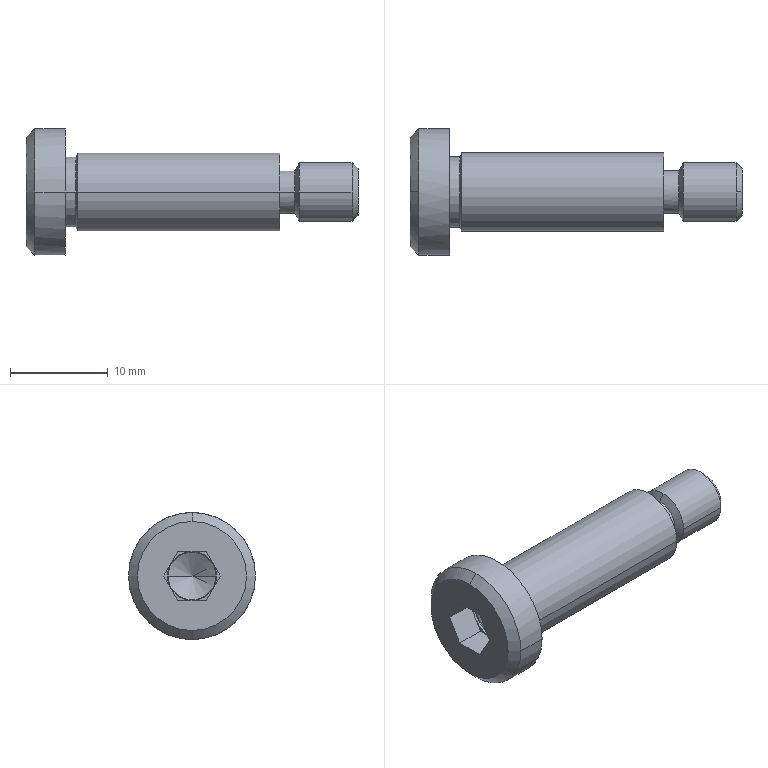Part | SolidWorks | features BaseBody 1 | 1 solid | 40 faces | box 34 x 13 x 13 mm | volume 1729 mm3 | plane 16 | cylinder 12 | cone 10 | spline 2 | commonest cylinder face diameters 4.4 x2 5 x2 6 x2 7.22 x2 8 x2 13 x2
STEP:
#1=CARTESIAN_POINT('',(-0.6825,-2.45,0.));
#2=VERTEX_POINT('',#1);
#3=CARTESIAN_POINT('',(-0.6825,2.45,0.));
#4=VERTEX_POINT('',#3);
#5=CARTESIAN_POINT('',(-0.6825,0.,0.));
#6=DIRECTION('',(-1.,0.,0.));
#7=DIRECTION('',(0.,1.,0.));
#8=AXIS2_PLACEMENT_3D('',#5,#6,#7);
#9=CIRCLE('',#8,2.45);
#10=EDGE_CURVE('',#2,#4,#9,.T.);
#11=ORIENTED_EDGE('',*,*,#10,.F.);
#12=CARTESIAN_POINT('',(-0.7691,-2.5,0.));
#13=VERTEX_POINT('',#12);
#14=CARTESIAN_POINT('',(-0.7691,-2.4,0.));
#15=DIRECTION('',(0.,0.,-1.));
#16=DIRECTION('',(0.,-1.,0.));
#17=AXIS2_PLACEMENT_3D('',#14,#15,#16);
#18=CIRCLE('',#17,0.1);
#19=EDGE_CURVE('',#2,#13,#18,.T.);
#20=ORIENTED_EDGE('',*,*,#19,.T.);
#21=CARTESIAN_POINT('',(-0.7691,2.5,0.));
#22=VERTEX_POINT('',#21);
#23=CARTESIAN_POINT('',(-0.7691,0.,0.));
#24=DIRECTION('',(-1.,0.,0.));
#25=DIRECTION('',(0.,1.,0.));
#26=AXIS2_PLACEMENT_3D('',#23,#24,#25);
#27=CIRCLE('',#26,2.5);
#28=EDGE_CURVE('',#13,#22,#27,.T.);
#29=ORIENTED_EDGE('',*,*,#28,.T.);
#30=CARTESIAN_POINT('',(-0.7691,2.4,0.));
#31=DIRECTION('',(0.,0.,1.));
#32=DIRECTION('',(0.,1.,0.));
#33=AXIS2_PLACEMENT_3D('',#30,#31,#32);
#34=CIRCLE('',#33,0.1);
#35=EDGE_CURVE('',#4,#22,#34,.T.);
#36=ORIENTED_EDGE('',*,*,#35,.F.);
#37=EDGE_LOOP('',(#11,#20,#29,#36));
#38=FACE_OUTER_BOUND('',#37,.T.);
#39=CARTESIAN_POINT('',(-0.6825,2.45,0.));
#40=CARTESIAN_POINT('',(-0.6825,2.45,4.9));
#41=CARTESIAN_POINT('',(-0.6825,-2.45,4.9));
#42=CARTESIAN_POINT('',(-0.6825,-2.45,0.));
#43=CARTESIAN_POINT('',(-0.7008,2.482,0.));
#44=CARTESIAN_POINT('',(-0.7008,2.482,4.963));
#45=CARTESIAN_POINT('',(-0.7008,-2.482,4.963));
#46=CARTESIAN_POINT('',(-0.7008,-2.482,0.));
#47=CARTESIAN_POINT('',(-0.7325,2.5,0.));
#48=CARTESIAN_POINT('',(-0.7325,2.5,5.));
#49=CARTESIAN_POINT('',(-0.7325,-2.5,5.));
#50=CARTESIAN_POINT('',(-0.7325,-2.5,0.));
#51=CARTESIAN_POINT('',(-0.7691,2.5,0.));
#52=CARTESIAN_POINT('',(-0.7691,2.5,5.));
#53=CARTESIAN_POINT('',(-0.7691,-2.5,5.));
#54=CARTESIAN_POINT('',(-0.7691,-2.5,0.));
#55=(BOUNDED_SURFACE()B_SPLINE_SURFACE(3,3,((#39,#40,#41,#42),(#43,#44,#45,#46),(#47,#48,#49,#50),(#51,#52,#53,#54)),.UNSPECIFIED.,.F.,.F.,.F.)B_SPLINE_SURFACE_WITH_KNOTS((4,4),(4,4),(0.,1.),(0.,1.),.UNSPECIFIED.)GEOMETRIC_REPRESENTATION_ITEM()RATIONAL_B_SPLINE_SURFACE(((1.,0.3333,0.3333,1.),(0.9107,0.3036,0.3036,0.9107),(0.9107,0.3036,0.3036,0.9107),(1.,0.3333,0.3333,1.)))REPRESENTATION_ITEM('')SURFACE());
#56=ADVANCED_FACE('',(#38),#55,.F.);
#57=CARTESIAN_POINT('',(1.3,4.,0.));
#58=VERTEX_POINT('',#57);
#59=CARTESIAN_POINT('',(1.3,-4.,0.));
#60=VERTEX_POINT('',#59);
#61=CARTESIAN_POINT('',(1.3,0.,0.));
#62=DIRECTION('',(1.,0.,0.));
#63=DIRECTION('',(0.,1.,0.));
#64=AXIS2_PLACEMENT_3D('',#61,#62,#63);
#65=CIRCLE('',#64,4.);
#66=EDGE_CURVE('',#58,#60,#65,.T.);
#67=ORIENTED_EDGE('',*,*,#66,.T.);
#68=CARTESIAN_POINT('',(22.,-4.,0.));
#69=VERTEX_POINT('',#68);
#70=CARTESIAN_POINT('',(500.,-4.,0.));
#71=DIRECTION('',(1.,0.,0.));
#72=VECTOR('',#71,1000.);
#73=LINE('',#70,#72);
#74=EDGE_CURVE('',#60,#69,#73,.T.);
#75=ORIENTED_EDGE('',*,*,#74,.T.);
#76=CARTESIAN_POINT('',(22.,4.,0.));
#77=VERTEX_POINT('',#76);
#78=CARTESIAN_POINT('',(22.,0.,0.));
#79=DIRECTION('',(-1.,0.,0.));
#80=DIRECTION('',(0.,1.,0.));
#81=AXIS2_PLACEMENT_3D('',#78,#79,#80);
#82=CIRCLE('',#81,4.);
#83=EDGE_CURVE('',#69,#77,#82,.T.);
#84=ORIENTED_EDGE('',*,*,#83,.T.);
#85=CARTESIAN_POINT('',(500.,4.,0.));
#86=DIRECTION('',(1.,0.,0.));
#87=VECTOR('',#86,1000.);
#88=LINE('',#85,#87);
#89=EDGE_CURVE('',#58,#77,#88,.T.);
#90=ORIENTED_EDGE('',*,*,#89,.F.);
#91=EDGE_LOOP('',(#67,#75,#84,#90));
#92=FACE_OUTER_BOUND('',#91,.T.);
#93=CARTESIAN_POINT('',(500.,0.,0.));
#94=DIRECTION('',(1.,0.,0.));
#95=DIRECTION('',(0.,1.,0.));
#96=AXIS2_PLACEMENT_3D('',#93,#94,#95);
#97=CYLINDRICAL_SURFACE('',#96,4.);
#98=ADVANCED_FACE('',(#92),#97,.T.);
#99=CARTESIAN_POINT('',(1.075,3.61,0.));
#100=VERTEX_POINT('',#99);
#101=CARTESIAN_POINT('',(1.075,-3.61,0.));
#102=VERTEX_POINT('',#101);
#103=CARTESIAN_POINT('',(1.075,0.,0.));
#104=DIRECTION('',(1.,0.,0.));
#105=DIRECTION('',(0.,1.,0.));
#106=AXIS2_PLACEMENT_3D('',#103,#104,#105);
#107=CIRCLE('',#106,3.61);
#108=EDGE_CURVE('',#100,#102,#107,.T.);
#109=ORIENTED_EDGE('',*,*,#108,.T.);
#110=CARTESIAN_POINT('',(1.3,-4.,0.));
#111=DIRECTION('',(0.5,-0.866,0.));
#112=VECTOR('',#111,1000.);
#113=LINE('',#110,#112);
#114=EDGE_CURVE('',#102,#60,#113,.T.);
#115=ORIENTED_EDGE('',*,*,#114,.T.);
#116=ORIENTED_EDGE('',*,*,#66,.F.);
#117=CARTESIAN_POINT('',(1.3,4.,0.));
#118=DIRECTION('',(0.5,0.866,0.));
#119=VECTOR('',#118,1000.);
#120=LINE('',#117,#119);
#121=EDGE_CURVE('',#100,#58,#120,.T.);
#122=ORIENTED_EDGE('',*,*,#121,.F.);
#123=EDGE_LOOP('',(#109,#115,#116,#122));
#124=FACE_OUTER_BOUND('',#123,.T.);
#125=CARTESIAN_POINT('',(1.3,0.,0.));
#126=DIRECTION('',(1.,0.,0.));
#127=DIRECTION('',(0.,1.,0.));
#128=AXIS2_PLACEMENT_3D('',#125,#126,#127);
#129=CONICAL_SURFACE('',#128,4.,1.047);
#130=ADVANCED_FACE('',(#124),#129,.T.);
#131=CARTESIAN_POINT('',(0.,3.61,0.));
#132=VERTEX_POINT('',#131);
#133=CARTESIAN_POINT('',(0.,-3.61,0.));
#134=VERTEX_POINT('',#133);
#135=CARTESIAN_POINT('',(0.,0.,0.));
#136=DIRECTION('',(1.,0.,0.));
#137=DIRECTION('',(0.,1.,0.));
#138=AXIS2_PLACEMENT_3D('',#135,#136,#137);
#139=CIRCLE('',#138,3.61);
#140=EDGE_CURVE('',#132,#134,#139,.T.);
#141=ORIENTED_EDGE('',*,*,#140,.T.);
#142=CARTESIAN_POINT('',(500.,-3.61,0.));
#143=DIRECTION('',(1.,0.,0.));
#144=VECTOR('',#143,1000.);
#145=LINE('',#142,#144);
#146=EDGE_CURVE('',#134,#102,#145,.T.);
#147=ORIENTED_EDGE('',*,*,#146,.T.);
#148=ORIENTED_EDGE('',*,*,#108,.F.);
#149=CARTESIAN_POINT('',(500.,3.61,0.));
#150=DIRECTION('',(1.,0.,0.));
#151=VECTOR('',#150,1000.);
#152=LINE('',#149,#151);
#153=EDGE_CURVE('',#132,#100,#152,.T.);
#154=ORIENTED_EDGE('',*,*,#153,.F.);
#155=EDGE_LOOP('',(#141,#147,#148,#154));
#156=FACE_OUTER_BOUND('',#155,.T.);
#157=CARTESIAN_POINT('',(500.,0.,0.));
#158=DIRECTION('',(1.,0.,0.));
#159=DIRECTION('',(0.,1.,0.));
#160=AXIS2_PLACEMENT_3D('',#157,#158,#159);
#161=CYLINDRICAL_SURFACE('',#160,3.61);
#162=ADVANCED_FACE('',(#156),#161,.T.);
#163=CARTESIAN_POINT('',(22.,2.2,0.));
#164=VERTEX_POINT('',#163);
#165=CARTESIAN_POINT('',(22.,-2.2,0.));
#166=VERTEX_POINT('',#165);
#167=CARTESIAN_POINT('',(22.,0.,0.));
#168=DIRECTION('',(1.,0.,0.));
#169=DIRECTION('',(0.,1.,0.));
#170=AXIS2_PLACEMENT_3D('',#167,#168,#169);
#171=CIRCLE('',#170,2.2);
#172=EDGE_CURVE('',#164,#166,#171,.T.);
#173=ORIENTED_EDGE('',*,*,#172,.T.);
#174=CARTESIAN_POINT('',(23.538,-2.2,0.));
#175=VERTEX_POINT('',#174);
#176=CARTESIAN_POINT('',(500.,-2.2,0.));
#177=DIRECTION('',(1.,0.,0.));
#178=VECTOR('',#177,1000.);
#179=LINE('',#176,#178);
#180=EDGE_CURVE('',#166,#175,#179,.T.);
#181=ORIENTED_EDGE('',*,*,#180,.T.);
#182=CARTESIAN_POINT('',(23.538,0.,2.2));
#183=VERTEX_POINT('',#182);
#184=CARTESIAN_POINT('',(23.538,0.,0.));
#185=DIRECTION('',(-1.,0.,0.));
#186=DIRECTION('',(0.,1.,0.));
#187=AXIS2_PLACEMENT_3D('',#184,#185,#186);
#188=CIRCLE('',#187,2.2);
#189=EDGE_CURVE('',#175,#183,#188,.T.);
#190=ORIENTED_EDGE('',*,*,#189,.T.);
#191=CARTESIAN_POINT('',(23.538,2.2,0.));
#192=VERTEX_POINT('',#191);
#193=CARTESIAN_POINT('',(23.538,0.,0.));
#194=DIRECTION('',(-1.,0.,0.));
#195=DIRECTION('',(0.,1.,0.));
#196=AXIS2_PLACEMENT_3D('',#193,#194,#195);
#197=CIRCLE('',#196,2.2);
#198=EDGE_CURVE('',#183,#192,#197,.T.);
#199=ORIENTED_EDGE('',*,*,#198,.T.);
#200=CARTESIAN_POINT('',(500.,2.2,0.));
#201=DIRECTION('',(1.,0.,0.));
#202=VECTOR('',#201,1000.);
#203=LINE('',#200,#202);
#204=EDGE_CURVE('',#164,#192,#203,.T.);
#205=ORIENTED_EDGE('',*,*,#204,.F.);
#206=EDGE_LOOP('',(#173,#181,#190,#199,#205));
#207=FACE_OUTER_BOUND('',#206,.T.);
#208=CARTESIAN_POINT('',(500.,0.,0.));
#209=DIRECTION('',(1.,0.,0.));
#210=DIRECTION('',(0.,1.,0.));
#211=AXIS2_PLACEMENT_3D('',#208,#209,#210);
#212=CYLINDRICAL_SURFACE('',#211,2.2);
#213=ADVANCED_FACE('',(#207),#212,.T.);
#214=ORIENTED_EDGE('',*,*,#198,.F.);
#215=CARTESIAN_POINT('',(24.,0.,3.));
#216=VERTEX_POINT('',#215);
#217=CARTESIAN_POINT('',(24.,0.,3.));
#218=DIRECTION('',(0.5,0.,0.866));
#219=VECTOR('',#218,1000.);
#220=LINE('',#217,#219);
#221=EDGE_CURVE('',#183,#216,#220,.T.);
#222=ORIENTED_EDGE('',*,*,#221,.T.);
#223=CARTESIAN_POINT('',(24.,3.,0.));
#224=VERTEX_POINT('',#223);
#225=CARTESIAN_POINT('',(24.,0.,0.));
#226=DIRECTION('',(-1.,0.,0.));
#227=DIRECTION('',(0.,1.,0.));
#228=AXIS2_PLACEMENT_3D('',#225,#226,#227);
#229=CIRCLE('',#228,3.);
#230=EDGE_CURVE('',#216,#224,#229,.T.);
#231=ORIENTED_EDGE('',*,*,#230,.T.);
#232=CARTESIAN_POINT('',(24.,0.,-3.));
#233=VERTEX_POINT('',#232);
#234=CARTESIAN_POINT('',(24.,0.,0.));
#235=DIRECTION('',(-1.,0.,0.));
#236=DIRECTION('',(0.,1.,0.));
#237=AXIS2_PLACEMENT_3D('',#234,#235,#236);
#238=CIRCLE('',#237,3.);
#239=EDGE_CURVE('',#224,#233,#238,.T.);
#240=ORIENTED_EDGE('',*,*,#239,.T.);
#241=CARTESIAN_POINT('',(23.538,0.,-2.2));
#242=VERTEX_POINT('',#241);
#243=CARTESIAN_POINT('',(24.,0.,-3.));
#244=DIRECTION('',(0.5,0.,-0.866));
#245=VECTOR('',#244,1000.);
#246=LINE('',#243,#245);
#247=EDGE_CURVE('',#242,#233,#246,.T.);
#248=ORIENTED_EDGE('',*,*,#247,.F.);
#249=CARTESIAN_POINT('',(23.538,0.,0.));
#250=DIRECTION('',(-1.,0.,0.));
#251=DIRECTION('',(0.,1.,0.));
#252=AXIS2_PLACEMENT_3D('',#249,#250,#251);
#253=CIRCLE('',#252,2.2);
#254=EDGE_CURVE('',#192,#242,#253,.T.);
#255=ORIENTED_EDGE('',*,*,#254,.F.);
#256=EDGE_LOOP('',(#214,#222,#231,#240,#248,#255));
#257=FACE_OUTER_BOUND('',#256,.T.);
#258=CARTESIAN_POINT('',(24.,0.,0.));
#259=DIRECTION('',(1.,0.,0.));
#260=DIRECTION('',(0.,0.,-1.));
#261=AXIS2_PLACEMENT_3D('',#258,#259,#260);
#262=CONICAL_SURFACE('',#261,3.,1.047);
#263=ADVANCED_FACE('',(#257),#262,.T.);
#264=CARTESIAN_POINT('',(-3.081,0.,6.5));
#265=VERTEX_POINT('',#264);
#266=CARTESIAN_POINT('',(-3.081,-6.5,0.));
#267=VERTEX_POINT('',#266);
#268=CARTESIAN_POINT('',(-3.081,0.,0.));
#269=DIRECTION('',(1.,0.,0.));
#270=DIRECTION('',(0.,1.,0.));
#271=AXIS2_PLACEMENT_3D('',#268,#269,#270);
#272=CIRCLE('',#271,6.5);
#273=EDGE_CURVE('',#265,#267,#272,.T.);
#274=ORIENTED_EDGE('',*,*,#273,.T.);
#275=CARTESIAN_POINT('',(0.,-6.5,0.));
#276=VERTEX_POINT('',#275);
#277=CARTESIAN_POINT('',(500.,-6.5,0.));
#278=DIRECTION('',(1.,0.,0.));
#279=VECTOR('',#278,1000.);
#280=LINE('',#277,#279);
#281=EDGE_CURVE('',#267,#276,#280,.T.);
#282=ORIENTED_EDGE('',*,*,#281,.T.);
#283=CARTESIAN_POINT('',(0.,6.5,0.));
#284=VERTEX_POINT('',#283);
#285=CARTESIAN_POINT('',(0.,0.,0.));
#286=DIRECTION('',(-1.,0.,0.));
#287=DIRECTION('',(0.,1.,0.));
#288=AXIS2_PLACEMENT_3D('',#285,#286,#287);
#289=CIRCLE('',#288,6.5);
#290=EDGE_CURVE('',#276,#284,#289,.T.);
#291=ORIENTED_EDGE('',*,*,#290,.T.);
#292=CARTESIAN_POINT('',(-3.081,6.5,0.));
#293=VERTEX_POINT('',#292);
#294=CARTESIAN_POINT('',(500.,6.5,0.));
#295=DIRECTION('',(1.,0.,0.));
#296=VECTOR('',#295,1000.);
#297=LINE('',#294,#296);
#298=EDGE_CURVE('',#293,#284,#297,.T.);
#299=ORIENTED_EDGE('',*,*,#298,.F.);
#300=CARTESIAN_POINT('',(-3.081,0.,0.));
#301=DIRECTION('',(1.,0.,0.));
#302=DIRECTION('',(0.,1.,0.));
#303=AXIS2_PLACEMENT_3D('',#300,#301,#302);
#304=CIRCLE('',#303,6.5);
#305=EDGE_CURVE('',#293,#265,#304,.T.);
#306=ORIENTED_EDGE('',*,*,#305,.T.);
#307=EDGE_LOOP('',(#274,#282,#291,#299,#306));
#308=FACE_OUTER_BOUND('',#307,.T.);
#309=CARTESIAN_POINT('',(500.,0.,0.));
#310=DIRECTION('',(1.,0.,0.));
#311=DIRECTION('',(0.,1.,0.));
#312=AXIS2_PLACEMENT_3D('',#309,#310,#311);
#313=CYLINDRICAL_SURFACE('',#312,6.5);
#314=ADVANCED_FACE('',(#308),#313,.T.);
#315=CARTESIAN_POINT('',(24.,-3.,0.));
#316=VERTEX_POINT('',#315);
#317=CARTESIAN_POINT('',(24.,0.,0.));
#318=DIRECTION('',(-1.,0.,0.));
#319=DIRECTION('',(0.,1.,0.));
#320=AXIS2_PLACEMENT_3D('',#317,#318,#319);
#321=CIRCLE('',#320,3.);
#322=EDGE_CURVE('',#316,#216,#321,.T.);
#323=ORIENTED_EDGE('',*,*,#322,.F.);
#324=CARTESIAN_POINT('',(29.386,-3.,0.));
#325=VERTEX_POINT('',#324);
#326=CARTESIAN_POINT('',(500.,-3.,0.));
#327=DIRECTION('',(1.,0.,0.));
#328=VECTOR('',#327,1000.);
#329=LINE('',#326,#328);
#330=EDGE_CURVE('',#316,#325,#329,.T.);
#331=ORIENTED_EDGE('',*,*,#330,.T.);
#332=CARTESIAN_POINT('',(29.386,0.,3.));
#333=VERTEX_POINT('',#332);
#334=CARTESIAN_POINT('',(29.386,0.,0.));
#335=DIRECTION('',(-1.,0.,0.));
#336=DIRECTION('',(0.,1.,0.));
#337=AXIS2_PLACEMENT_3D('',#334,#335,#336);
#338=CIRCLE('',#337,3.);
#339=EDGE_CURVE('',#325,#333,#338,.T.);
#340=ORIENTED_EDGE('',*,*,#339,.T.);
#341=CARTESIAN_POINT('',(29.386,3.,0.));
#342=VERTEX_POINT('',#341);
#343=CARTESIAN_POINT('',(29.386,0.,0.));
#344=DIRECTION('',(-1.,0.,0.));
#345=DIRECTION('',(0.,1.,0.));
#346=AXIS2_PLACEMENT_3D('',#343,#344,#345);
#347=CIRCLE('',#346,3.);
#348=EDGE_CURVE('',#333,#342,#347,.T.);
#349=ORIENTED_EDGE('',*,*,#348,.T.);
#350=CARTESIAN_POINT('',(500.,3.,0.));
#351=DIRECTION('',(1.,0.,0.));
#352=VECTOR('',#351,1000.);
#353=LINE('',#350,#352);
#354=EDGE_CURVE('',#224,#342,#353,.T.);
#355=ORIENTED_EDGE('',*,*,#354,.F.);
#356=ORIENTED_EDGE('',*,*,#230,.F.);
#357=EDGE_LOOP('',(#323,#331,#340,#349,#355,#356));
#358=FACE_OUTER_BOUND('',#357,.T.);
#359=CARTESIAN_POINT('',(500.,0.,0.));
#360=DIRECTION('',(1.,0.,0.));
#361=DIRECTION('',(0.,1.,0.));
#362=AXIS2_PLACEMENT_3D('',#359,#360,#361);
#363=CYLINDRICAL_SURFACE('',#362,3.);
#364=ADVANCED_FACE('',(#358),#363,.T.);
#365=CARTESIAN_POINT('',(-4.,0.,-5.581));
#366=VERTEX_POINT('',#365);
#367=CARTESIAN_POINT('',(-4.,0.,5.581));
#368=VERTEX_POINT('',#367);
#369=CARTESIAN_POINT('',(-4.,0.,0.));
#370=DIRECTION('',(1.,0.,0.));
#371=DIRECTION('',(0.,0.,-1.));
#372=AXIS2_PLACEMENT_3D('',#369,#370,#371);
#373=CIRCLE('',#372,5.581);
#374=EDGE_CURVE('',#366,#368,#373,.T.);
#375=ORIENTED_EDGE('',*,*,#374,.T.);
#376=CARTESIAN_POINT('',(-3.081,0.,6.5));
#377=DIRECTION('',(0.7071,0.,0.7071));
#378=VECTOR('',#377,1000.);
#379=LINE('',#376,#378);
#380=EDGE_CURVE('',#368,#265,#379,.T.);
#381=ORIENTED_EDGE('',*,*,#380,.T.);
#382=ORIENTED_EDGE('',*,*,#305,.F.);
#383=CARTESIAN_POINT('',(-3.081,0.,-6.5));
#384=VERTEX_POINT('',#383);
#385=CARTESIAN_POINT('',(-3.081,0.,0.));
#386=DIRECTION('',(1.,0.,0.));
#387=DIRECTION('',(0.,1.,0.));
#388=AXIS2_PLACEMENT_3D('',#385,#386,#387);
#389=CIRCLE('',#388,6.5);
#390=EDGE_CURVE('',#384,#293,#389,.T.);
#391=ORIENTED_EDGE('',*,*,#390,.F.);
#392=CARTESIAN_POINT('',(-3.081,0.,-6.5));
#393=DIRECTION('',(0.7071,0.,-0.7071));
#394=VECTOR('',#393,1000.);
#395=LINE('',#392,#394);
#396=EDGE_CURVE('',#366,#384,#395,.T.);
#397=ORIENTED_EDGE('',*,*,#396,.F.);
#398=EDGE_LOOP('',(#375,#381,#382,#391,#397));
#399=FACE_OUTER_BOUND('',#398,.T.);
#400=CARTESIAN_POINT('',(-3.081,0.,0.));
#401=DIRECTION('',(1.,0.,0.));
#402=DIRECTION('',(0.,0.,-1.));
#403=AXIS2_PLACEMENT_3D('',#400,#401,#402);
#404=CONICAL_SURFACE('',#403,6.5,0.7854);
#405=ADVANCED_FACE('',(#399),#404,.T.);
#406=CARTESIAN_POINT('',(30.,0.,2.387));
#407=VERTEX_POINT('',#406);
#408=CARTESIAN_POINT('',(30.,0.,-2.387));
#409=VERTEX_POINT('',#408);
#410=CARTESIAN_POINT('',(30.,0.,0.));
#411=DIRECTION('',(-1.,0.,0.));
#412=DIRECTION('',(0.,0.,1.));
#413=AXIS2_PLACEMENT_3D('',#410,#411,#412);
#414=CIRCLE('',#413,2.387);
#415=EDGE_CURVE('',#407,#409,#414,.T.);
#416=ORIENTED_EDGE('',*,*,#415,.T.);
#417=CARTESIAN_POINT('',(29.386,0.,-3.));
#418=VERTEX_POINT('',#417);
#419=CARTESIAN_POINT('',(29.387,0.,-3.));
#420=DIRECTION('',(-0.7071,0.,-0.7071));
#421=VECTOR('',#420,1000.);
#422=LINE('',#419,#421);
#423=EDGE_CURVE('',#409,#418,#422,.T.);
#424=ORIENTED_EDGE('',*,*,#423,.T.);
#425=CARTESIAN_POINT('',(29.386,0.,0.));
#426=DIRECTION('',(-1.,0.,0.));
#427=DIRECTION('',(0.,1.,0.));
#428=AXIS2_PLACEMENT_3D('',#425,#426,#427);
#429=CIRCLE('',#428,3.);
#430=EDGE_CURVE('',#342,#418,#429,.T.);
#431=ORIENTED_EDGE('',*,*,#430,.F.);
#432=ORIENTED_EDGE('',*,*,#348,.F.);
#433=CARTESIAN_POINT('',(29.387,0.,3.));
#434=DIRECTION('',(-0.7071,0.,0.7071));
#435=VECTOR('',#434,1000.);
#436=LINE('',#433,#435);
#437=EDGE_CURVE('',#407,#333,#436,.T.);
#438=ORIENTED_EDGE('',*,*,#437,.F.);
#439=EDGE_LOOP('',(#416,#424,#431,#432,#438));
#440=FACE_OUTER_BOUND('',#439,.T.);
#441=CARTESIAN_POINT('',(29.387,0.,0.));
#442=DIRECTION('',(-1.,0.,0.));
#443=DIRECTION('',(0.,0.,1.));
#444=AXIS2_PLACEMENT_3D('',#441,#442,#443);
#445=CONICAL_SURFACE('',#444,3.,0.7854);
#446=ADVANCED_FACE('',(#440),#445,.T.);
#447=CARTESIAN_POINT('',(-1.,-2.5,0.));
#448=VERTEX_POINT('',#447);
#449=CARTESIAN_POINT('',(-1.,-2.165,-1.25));
#450=VERTEX_POINT('',#449);
#451=CARTESIAN_POINT('',(-1.,0.,0.));
#452=DIRECTION('',(1.,0.,0.));
#453=DIRECTION('',(0.,1.,0.));
#454=AXIS2_PLACEMENT_3D('',#451,#452,#453);
#455=CIRCLE('',#454,2.5);
#456=EDGE_CURVE('',#448,#450,#455,.T.);
#457=ORIENTED_EDGE('',*,*,#456,.F.);
#458=CARTESIAN_POINT('',(500.,-2.5,0.));
#459=DIRECTION('',(1.,0.,0.));
#460=VECTOR('',#459,1000.);
#461=LINE('',#458,#460);
#462=EDGE_CURVE('',#448,#13,#461,.T.);
#463=ORIENTED_EDGE('',*,*,#462,.T.);
#464=CARTESIAN_POINT('',(-0.7691,0.,0.));
#465=DIRECTION('',(-1.,0.,0.));
#466=DIRECTION('',(0.,1.,0.));
#467=AXIS2_PLACEMENT_3D('',#464,#465,#466);
#468=CIRCLE('',#467,2.5);
#469=EDGE_CURVE('',#22,#13,#468,.T.);
#470=ORIENTED_EDGE('',*,*,#469,.F.);
#471=CARTESIAN_POINT('',(-1.,2.5,0.));
#472=VERTEX_POINT('',#471);
#473=CARTESIAN_POINT('',(500.,2.5,0.));
#474=DIRECTION('',(1.,0.,0.));
#475=VECTOR('',#474,1000.);
#476=LINE('',#473,#475);
#477=EDGE_CURVE('',#472,#22,#476,.T.);
#478=ORIENTED_EDGE('',*,*,#477,.F.);
#479=CARTESIAN_POINT('',(-1.,2.165,-1.25));
#480=VERTEX_POINT('',#479);
#481=CARTESIAN_POINT('',(-1.,0.,0.));
#482=DIRECTION('',(1.,0.,0.));
#483=DIRECTION('',(0.,1.,0.));
#484=AXIS2_PLACEMENT_3D('',#481,#482,#483);
#485=CIRCLE('',#484,2.5);
#486=EDGE_CURVE('',#480,#472,#485,.T.);
#487=ORIENTED_EDGE('',*,*,#486,.F.);
#488=CARTESIAN_POINT('',(-1.,0.,-2.5));
#489=VERTEX_POINT('',#488);
#490=CARTESIAN_POINT('',(-1.,0.,0.));
#491=DIRECTION('',(1.,0.,0.));
#492=DIRECTION('',(0.,1.,0.));
#493=AXIS2_PLACEMENT_3D('',#490,#491,#492);
#494=CIRCLE('',#493,2.5);
#495=EDGE_CURVE('',#489,#480,#494,.T.);
#496=ORIENTED_EDGE('',*,*,#495,.F.);
#497=CARTESIAN_POINT('',(-1.,0.,0.));
#498=DIRECTION('',(1.,0.,0.));
#499=DIRECTION('',(0.,1.,0.));
#500=AXIS2_PLACEMENT_3D('',#497,#498,#499);
#501=CIRCLE('',#500,2.5);
#502=EDGE_CURVE('',#450,#489,#501,.T.);
#503=ORIENTED_EDGE('',*,*,#502,.F.);
#504=EDGE_LOOP('',(#457,#463,#470,#478,#487,#496,#503));
#505=FACE_OUTER_BOUND('',#504,.T.);
#506=CARTESIAN_POINT('',(500.,0.,0.));
#507=DIRECTION('',(1.,0.,0.));
#508=DIRECTION('',(0.,1.,0.));
#509=AXIS2_PLACEMENT_3D('',#506,#507,#508);
#510=CYLINDRICAL_SURFACE('',#509,2.5);
#511=ADVANCED_FACE('',(#505),#510,.F.);
#512=CARTESIAN_POINT('',(0.7321,0.,0.));
#513=VERTEX_POINT('',#512);
#514=CARTESIAN_POINT('',(-0.6825,-2.45,0.));
#515=DIRECTION('',(-0.5,-0.866,0.));
#516=VECTOR('',#515,1000.);
#517=LINE('',#514,#516);
#518=EDGE_CURVE('',#513,#2,#517,.T.);
#519=ORIENTED_EDGE('',*,*,#518,.F.);
#520=CARTESIAN_POINT('',(-0.6825,2.45,0.));
#521=DIRECTION('',(-0.5,0.866,0.));
#522=VECTOR('',#521,1000.);
#523=LINE('',#520,#522);
#524=EDGE_CURVE('',#513,#4,#523,.T.);
#525=ORIENTED_EDGE('',*,*,#524,.T.);
#526=CARTESIAN_POINT('',(-0.6825,0.,0.));
#527=DIRECTION('',(-1.,0.,0.));
#528=DIRECTION('',(0.,1.,0.));
#529=AXIS2_PLACEMENT_3D('',#526,#527,#528);
#530=CIRCLE('',#529,2.45);
#531=EDGE_CURVE('',#4,#2,#530,.T.);
#532=ORIENTED_EDGE('',*,*,#531,.T.);
#533=EDGE_LOOP('',(#519,#525,#532));
#534=FACE_OUTER_BOUND('',#533,.T.);
#535=CARTESIAN_POINT('',(-0.6825,0.,0.));
#536=DIRECTION('',(-1.,0.,0.));
#537=DIRECTION('',(0.,-1.,0.));
#538=AXIS2_PLACEMENT_3D('',#535,#536,#537);
#539=CONICAL_SURFACE('',#538,2.45,1.047);
#540=ADVANCED_FACE('',(#534),#539,.F.);
#541=ORIENTED_EDGE('',*,*,#74,.F.);
#542=CARTESIAN_POINT('',(1.3,0.,0.));
#543=DIRECTION('',(1.,0.,0.));
#544=DIRECTION('',(0.,1.,0.));
#545=AXIS2_PLACEMENT_3D('',#542,#543,#544);
#546=CIRCLE('',#545,4.);
#547=EDGE_CURVE('',#60,#58,#546,.T.);
#548=ORIENTED_EDGE('',*,*,#547,.T.);
#549=ORIENTED_EDGE('',*,*,#89,.T.);
#550=CARTESIAN_POINT('',(22.,0.,0.));
#551=DIRECTION('',(-1.,0.,0.));
#552=DIRECTION('',(0.,1.,0.));
#553=AXIS2_PLACEMENT_3D('',#550,#551,#552);
#554=CIRCLE('',#553,4.);
#555=EDGE_CURVE('',#77,#69,#554,.T.);
#556=ORIENTED_EDGE('',*,*,#555,.T.);
#557=EDGE_LOOP('',(#541,#548,#549,#556));
#558=FACE_OUTER_BOUND('',#557,.T.);
#559=CARTESIAN_POINT('',(500.,0.,0.));
#560=DIRECTION('',(1.,0.,0.));
#561=DIRECTION('',(0.,1.,0.));
#562=AXIS2_PLACEMENT_3D('',#559,#560,#561);
#563=CYLINDRICAL_SURFACE('',#562,4.);
#564=ADVANCED_FACE('',(#558),#563,.T.);
#565=ORIENTED_EDGE('',*,*,#114,.F.);
#566=CARTESIAN_POINT('',(1.075,0.,0.));
#567=DIRECTION('',(1.,0.,0.));
#568=DIRECTION('',(0.,1.,0.));
#569=AXIS2_PLACEMENT_3D('',#566,#567,#568);
#570=CIRCLE('',#569,3.61);
#571=EDGE_CURVE('',#102,#100,#570,.T.);
#572=ORIENTED_EDGE('',*,*,#571,.T.);
#573=ORIENTED_EDGE('',*,*,#121,.T.);
#574=ORIENTED_EDGE('',*,*,#547,.F.);
#575=EDGE_LOOP('',(#565,#572,#573,#574));
#576=FACE_OUTER_BOUND('',#575,.T.);
#577=CARTESIAN_POINT('',(1.3,0.,0.));
#578=DIRECTION('',(1.,0.,0.));
#579=DIRECTION('',(0.,1.,0.));
#580=AXIS2_PLACEMENT_3D('',#577,#578,#579);
#581=CONICAL_SURFACE('',#580,4.,1.047);
#582=ADVANCED_FACE('',(#576),#581,.T.);
#583=ORIENTED_EDGE('',*,*,#555,.F.);
#584=ORIENTED_EDGE('',*,*,#83,.F.);
#585=EDGE_LOOP('',(#583,#584));
#586=FACE_OUTER_BOUND('',#585,.T.);
#587=ORIENTED_EDGE('',*,*,#172,.F.);
#588=CARTESIAN_POINT('',(22.,0.,0.));
#589=DIRECTION('',(1.,0.,0.));
#590=DIRECTION('',(0.,1.,0.));
#591=AXIS2_PLACEMENT_3D('',#588,#589,#590);
#592=CIRCLE('',#591,2.2);
#593=EDGE_CURVE('',#166,#164,#592,.T.);
#594=ORIENTED_EDGE('',*,*,#593,.F.);
#595=EDGE_LOOP('',(#587,#594));
#596=FACE_BOUND('',#595,.T.);
#597=CARTESIAN_POINT('',(22.,4.,0.));
#598=DIRECTION('',(-1.,0.,0.));
#599=DIRECTION('',(0.,-1.,0.));
#600=AXIS2_PLACEMENT_3D('',#597,#598,#599);
#601=PLANE('',#600);
#602=ADVANCED_FACE('',(#586,#596),#601,.F.);
#603=ORIENTED_EDGE('',*,*,#146,.F.);
#604=CARTESIAN_POINT('',(0.,0.,0.));
#605=DIRECTION('',(1.,0.,0.));
#606=DIRECTION('',(0.,1.,0.));
#607=AXIS2_PLACEMENT_3D('',#604,#605,#606);
#608=CIRCLE('',#607,3.61);
#609=EDGE_CURVE('',#134,#132,#608,.T.);
#610=ORIENTED_EDGE('',*,*,#609,.T.);
#611=ORIENTED_EDGE('',*,*,#153,.T.);
#612=ORIENTED_EDGE('',*,*,#571,.F.);
#613=EDGE_LOOP('',(#603,#610,#611,#612));
#614=FACE_OUTER_BOUND('',#613,.T.);
#615=CARTESIAN_POINT('',(500.,0.,0.));
#616=DIRECTION('',(1.,0.,0.));
#617=DIRECTION('',(0.,1.,0.));
#618=AXIS2_PLACEMENT_3D('',#615,#616,#617);
#619=CYLINDRICAL_SURFACE('',#618,3.61);
#620=ADVANCED_FACE('',(#614),#619,.T.);
#621=ORIENTED_EDGE('',*,*,#180,.F.);
#622=ORIENTED_EDGE('',*,*,#593,.T.);
#623=ORIENTED_EDGE('',*,*,#204,.T.);
#624=ORIENTED_EDGE('',*,*,#254,.T.);
#625=CARTESIAN_POINT('',(23.538,0.,0.));
#626=DIRECTION('',(-1.,0.,0.));
#627=DIRECTION('',(0.,1.,0.));
#628=AXIS2_PLACEMENT_3D('',#625,#626,#627);
#629=CIRCLE('',#628,2.2);
#630=EDGE_CURVE('',#242,#175,#629,.T.);
#631=ORIENTED_EDGE('',*,*,#630,.T.);
#632=EDGE_LOOP('',(#621,#622,#623,#624,#631));
#633=FACE_OUTER_BOUND('',#632,.T.);
#634=CARTESIAN_POINT('',(500.,0.,0.));
#635=DIRECTION('',(1.,0.,0.));
#636=DIRECTION('',(0.,1.,0.));
#637=AXIS2_PLACEMENT_3D('',#634,#635,#636);
#638=CYLINDRICAL_SURFACE('',#637,2.2);
#639=ADVANCED_FACE('',(#633),#638,.T.);
#640=CARTESIAN_POINT('',(0.,0.,0.));
#641=DIRECTION('',(-1.,0.,0.));
#642=DIRECTION('',(0.,1.,0.));
#643=AXIS2_PLACEMENT_3D('',#640,#641,#642);
#644=CIRCLE('',#643,6.5);
#645=EDGE_CURVE('',#284,#276,#644,.T.);
#646=ORIENTED_EDGE('',*,*,#645,.F.);
#647=ORIENTED_EDGE('',*,*,#290,.F.);
#648=EDGE_LOOP('',(#646,#647));
#649=FACE_OUTER_BOUND('',#648,.T.);
#650=ORIENTED_EDGE('',*,*,#140,.F.);
#651=ORIENTED_EDGE('',*,*,#609,.F.);
#652=EDGE_LOOP('',(#650,#651));
#653=FACE_BOUND('',#652,.T.);
#654=CARTESIAN_POINT('',(0.,6.5,0.));
#655=DIRECTION('',(-1.,0.,0.));
#656=DIRECTION('',(0.,-1.,0.));
#657=AXIS2_PLACEMENT_3D('',#654,#655,#656);
#658=PLANE('',#657);
#659=ADVANCED_FACE('',(#649,#653),#658,.F.);
#660=ORIENTED_EDGE('',*,*,#221,.F.);
#661=ORIENTED_EDGE('',*,*,#189,.F.);
#662=ORIENTED_EDGE('',*,*,#630,.F.);
#663=ORIENTED_EDGE('',*,*,#247,.T.);
#664=CARTESIAN_POINT('',(24.,0.,0.));
#665=DIRECTION('',(-1.,0.,0.));
#666=DIRECTION('',(0.,1.,0.));
#667=AXIS2_PLACEMENT_3D('',#664,#665,#666);
#668=CIRCLE('',#667,3.);
#669=EDGE_CURVE('',#233,#316,#668,.T.);
#670=ORIENTED_EDGE('',*,*,#669,.T.);
#671=ORIENTED_EDGE('',*,*,#322,.T.);
#672=EDGE_LOOP('',(#660,#661,#662,#663,#670,#671));
#673=FACE_OUTER_BOUND('',#672,.T.);
#674=CARTESIAN_POINT('',(24.,0.,0.));
#675=DIRECTION('',(1.,0.,0.));
#676=DIRECTION('',(0.,0.,-1.));
#677=AXIS2_PLACEMENT_3D('',#674,#675,#676);
#678=CONICAL_SURFACE('',#677,3.,1.047);
#679=ADVANCED_FACE('',(#673),#678,.T.);
#680=ORIENTED_EDGE('',*,*,#281,.F.);
#681=CARTESIAN_POINT('',(-3.081,0.,0.));
#682=DIRECTION('',(1.,0.,0.));
#683=DIRECTION('',(0.,1.,0.));
#684=AXIS2_PLACEMENT_3D('',#681,#682,#683);
#685=CIRCLE('',#684,6.5);
#686=EDGE_CURVE('',#267,#384,#685,.T.);
#687=ORIENTED_EDGE('',*,*,#686,.T.);
#688=ORIENTED_EDGE('',*,*,#390,.T.);
#689=ORIENTED_EDGE('',*,*,#298,.T.);
#690=ORIENTED_EDGE('',*,*,#645,.T.);
#691=EDGE_LOOP('',(#680,#687,#688,#689,#690));
#692=FACE_OUTER_BOUND('',#691,.T.);
#693=CARTESIAN_POINT('',(500.,0.,0.));
#694=DIRECTION('',(1.,0.,0.));
#695=DIRECTION('',(0.,1.,0.));
#696=AXIS2_PLACEMENT_3D('',#693,#694,#695);
#697=CYLINDRICAL_SURFACE('',#696,6.5);
#698=ADVANCED_FACE('',(#692),#697,.T.);
#699=ORIENTED_EDGE('',*,*,#330,.F.);
#700=ORIENTED_EDGE('',*,*,#669,.F.);
#701=ORIENTED_EDGE('',*,*,#239,.F.);
#702=ORIENTED_EDGE('',*,*,#354,.T.);
#703=ORIENTED_EDGE('',*,*,#430,.T.);
#704=CARTESIAN_POINT('',(29.386,0.,0.));
#705=DIRECTION('',(-1.,0.,0.));
#706=DIRECTION('',(0.,1.,0.));
#707=AXIS2_PLACEMENT_3D('',#704,#705,#706);
#708=CIRCLE('',#707,3.);
#709=EDGE_CURVE('',#418,#325,#708,.T.);
#710=ORIENTED_EDGE('',*,*,#709,.T.);
#711=EDGE_LOOP('',(#699,#700,#701,#702,#703,#710));
#712=FACE_OUTER_BOUND('',#711,.T.);
#713=CARTESIAN_POINT('',(500.,0.,0.));
#714=DIRECTION('',(1.,0.,0.));
#715=DIRECTION('',(0.,1.,0.));
#716=AXIS2_PLACEMENT_3D('',#713,#714,#715);
#717=CYLINDRICAL_SURFACE('',#716,3.);
#718=ADVANCED_FACE('',(#712),#717,.T.);
#719=ORIENTED_EDGE('',*,*,#380,.F.);
#720=CARTESIAN_POINT('',(-4.,0.,0.));
#721=DIRECTION('',(1.,0.,0.));
#722=DIRECTION('',(0.,0.,-1.));
#723=AXIS2_PLACEMENT_3D('',#720,#721,#722);
#724=CIRCLE('',#723,5.581);
#725=EDGE_CURVE('',#368,#366,#724,.T.);
#726=ORIENTED_EDGE('',*,*,#725,.T.);
#727=ORIENTED_EDGE('',*,*,#396,.T.);
#728=ORIENTED_EDGE('',*,*,#686,.F.);
#729=ORIENTED_EDGE('',*,*,#273,.F.);
#730=EDGE_LOOP('',(#719,#726,#727,#728,#729));
#731=FACE_OUTER_BOUND('',#730,.T.);
#732=CARTESIAN_POINT('',(-3.081,0.,0.));
#733=DIRECTION('',(1.,0.,0.));
#734=DIRECTION('',(0.,0.,-1.));
#735=AXIS2_PLACEMENT_3D('',#732,#733,#734);
#736=CONICAL_SURFACE('',#735,6.5,0.7854);
#737=ADVANCED_FACE('',(#731),#736,.T.);
#738=ORIENTED_EDGE('',*,*,#423,.F.);
#739=CARTESIAN_POINT('',(30.,0.,0.));
#740=DIRECTION('',(-1.,0.,0.));
#741=DIRECTION('',(0.,0.,1.));
#742=AXIS2_PLACEMENT_3D('',#739,#740,#741);
#743=CIRCLE('',#742,2.387);
#744=EDGE_CURVE('',#409,#407,#743,.T.);
#745=ORIENTED_EDGE('',*,*,#744,.T.);
#746=ORIENTED_EDGE('',*,*,#437,.T.);
#747=ORIENTED_EDGE('',*,*,#339,.F.);
#748=ORIENTED_EDGE('',*,*,#709,.F.);
#749=EDGE_LOOP('',(#738,#745,#746,#747,#748));
#750=FACE_OUTER_BOUND('',#749,.T.);
#751=CARTESIAN_POINT('',(29.387,0.,0.));
#752=DIRECTION('',(-1.,0.,0.));
#753=DIRECTION('',(0.,0.,1.));
#754=AXIS2_PLACEMENT_3D('',#751,#752,#753);
#755=CONICAL_SURFACE('',#754,3.,0.7854);
#756=ADVANCED_FACE('',(#750),#755,.T.);
#757=CARTESIAN_POINT('',(-4.,1.443,-2.5));
#758=VERTEX_POINT('',#757);
#759=CARTESIAN_POINT('',(-4.,-1.443,-2.5));
#760=VERTEX_POINT('',#759);
#761=CARTESIAN_POINT('',(-4.,2.5,-2.5));
#762=DIRECTION('',(0.,-1.,0.));
#763=VECTOR('',#762,1000.);
#764=LINE('',#761,#763);
#765=EDGE_CURVE('',#758,#760,#764,.T.);
#766=ORIENTED_EDGE('',*,*,#765,.F.);
#767=CARTESIAN_POINT('',(-4.,2.887,0.));
#768=VERTEX_POINT('',#767);
#769=CARTESIAN_POINT('',(-4.,2.887,0.));
#770=DIRECTION('',(0.,-0.5,-0.866));
#771=VECTOR('',#770,1000.);
#772=LINE('',#769,#771);
#773=EDGE_CURVE('',#768,#758,#772,.T.);
#774=ORIENTED_EDGE('',*,*,#773,.F.);
#775=CARTESIAN_POINT('',(-4.,1.443,2.5));
#776=VERTEX_POINT('',#775);
#777=CARTESIAN_POINT('',(-4.,1.443,2.5));
#778=DIRECTION('',(0.,0.5,-0.866));
#779=VECTOR('',#778,1000.);
#780=LINE('',#777,#779);
#781=EDGE_CURVE('',#776,#768,#780,.T.);
#782=ORIENTED_EDGE('',*,*,#781,.F.);
#783=CARTESIAN_POINT('',(-4.,-1.443,2.5));
#784=VERTEX_POINT('',#783);
#785=CARTESIAN_POINT('',(-4.,2.5,2.5));
#786=DIRECTION('',(0.,1.,0.));
#787=VECTOR('',#786,1000.);
#788=LINE('',#785,#787);
#789=EDGE_CURVE('',#784,#776,#788,.T.);
#790=ORIENTED_EDGE('',*,*,#789,.F.);
#791=CARTESIAN_POINT('',(-4.,-2.887,0.));
#792=VERTEX_POINT('',#791);
#793=CARTESIAN_POINT('',(-4.,-2.887,0.));
#794=DIRECTION('',(0.,0.5,0.866));
#795=VECTOR('',#794,1000.);
#796=LINE('',#793,#795);
#797=EDGE_CURVE('',#792,#784,#796,.T.);
#798=ORIENTED_EDGE('',*,*,#797,.F.);
#799=CARTESIAN_POINT('',(-4.,-1.443,-2.5));
#800=DIRECTION('',(0.,-0.5,0.866));
#801=VECTOR('',#800,1000.);
#802=LINE('',#799,#801);
#803=EDGE_CURVE('',#760,#792,#802,.T.);
#804=ORIENTED_EDGE('',*,*,#803,.F.);
#805=EDGE_LOOP('',(#766,#774,#782,#790,#798,#804));
#806=FACE_BOUND('',#805,.T.);
#807=ORIENTED_EDGE('',*,*,#374,.F.);
#808=ORIENTED_EDGE('',*,*,#725,.F.);
#809=EDGE_LOOP('',(#807,#808));
#810=FACE_OUTER_BOUND('',#809,.T.);
#811=CARTESIAN_POINT('',(-4.,2.5,0.));
#812=DIRECTION('',(1.,0.,0.));
#813=DIRECTION('',(0.,1.,0.));
#814=AXIS2_PLACEMENT_3D('',#811,#812,#813);
#815=PLANE('',#814);
#816=ADVANCED_FACE('',(#806,#810),#815,.F.);
#817=ORIENTED_EDGE('',*,*,#415,.F.);
#818=ORIENTED_EDGE('',*,*,#744,.F.);
#819=EDGE_LOOP('',(#817,#818));
#820=FACE_OUTER_BOUND('',#819,.T.);
#821=CARTESIAN_POINT('',(30.,2.386,0.));
#822=DIRECTION('',(-1.,0.,0.));
#823=DIRECTION('',(0.,-1.,0.));
#824=AXIS2_PLACEMENT_3D('',#821,#822,#823);
#825=PLANE('',#824);
#826=ADVANCED_FACE('',(#820),#825,.F.);
#827=ORIENTED_EDGE('',*,*,#803,.T.);
#828=CARTESIAN_POINT('',(-1.,-2.887,0.));
#829=VERTEX_POINT('',#828);
#830=CARTESIAN_POINT('',(-1.,-2.887,0.));
#831=DIRECTION('',(1.,0.,0.));
#832=VECTOR('',#831,1000.);
#833=LINE('',#830,#832);
#834=EDGE_CURVE('',#792,#829,#833,.T.);
#835=ORIENTED_EDGE('',*,*,#834,.T.);
#836=CARTESIAN_POINT('',(-1.,-2.887,0.));
#837=DIRECTION('',(0.,0.5,-0.866));
#838=VECTOR('',#837,1000.);
#839=LINE('',#836,#838);
#840=EDGE_CURVE('',#829,#450,#839,.T.);
#841=ORIENTED_EDGE('',*,*,#840,.T.);
#842=CARTESIAN_POINT('',(-1.,-1.443,-2.5));
#843=VERTEX_POINT('',#842);
#844=CARTESIAN_POINT('',(-1.,-2.165,-1.25));
#845=DIRECTION('',(0.,0.5,-0.866));
#846=VECTOR('',#845,1000.);
#847=LINE('',#844,#846);
#848=EDGE_CURVE('',#450,#843,#847,.T.);
#849=ORIENTED_EDGE('',*,*,#848,.T.);
#850=CARTESIAN_POINT('',(-1.,-1.443,-2.5));
#851=DIRECTION('',(-1.,0.,0.));
#852=VECTOR('',#851,1000.);
#853=LINE('',#850,#852);
#854=EDGE_CURVE('',#843,#760,#853,.T.);
#855=ORIENTED_EDGE('',*,*,#854,.T.);
#856=EDGE_LOOP('',(#827,#835,#841,#849,#855));
#857=FACE_OUTER_BOUND('',#856,.T.);
#858=CARTESIAN_POINT('',(-1.,-2.887,0.));
#859=DIRECTION('',(0.,0.866,0.5));
#860=DIRECTION('',(0.,-0.5,0.866));
#861=AXIS2_PLACEMENT_3D('',#858,#859,#860);
#862=PLANE('',#861);
#863=ADVANCED_FACE('',(#857),#862,.T.);
#864=ORIENTED_EDGE('',*,*,#765,.T.);
#865=ORIENTED_EDGE('',*,*,#854,.F.);
#866=CARTESIAN_POINT('',(-1.,0.,-2.5));
#867=DIRECTION('',(0.,1.,0.));
#868=VECTOR('',#867,1000.);
#869=LINE('',#866,#868);
#870=EDGE_CURVE('',#843,#489,#869,.T.);
#871=ORIENTED_EDGE('',*,*,#870,.T.);
#872=CARTESIAN_POINT('',(-1.,1.443,-2.5));
#873=VERTEX_POINT('',#872);
#874=CARTESIAN_POINT('',(-1.,0.,-2.5));
#875=DIRECTION('',(0.,1.,0.));
#876=VECTOR('',#875,1000.);
#877=LINE('',#874,#876);
#878=EDGE_CURVE('',#489,#873,#877,.T.);
#879=ORIENTED_EDGE('',*,*,#878,.T.);
#880=CARTESIAN_POINT('',(-1.,1.443,-2.5));
#881=DIRECTION('',(-1.,0.,0.));
#882=VECTOR('',#881,1000.);
#883=LINE('',#880,#882);
#884=EDGE_CURVE('',#873,#758,#883,.T.);
#885=ORIENTED_EDGE('',*,*,#884,.T.);
#886=EDGE_LOOP('',(#864,#865,#871,#879,#885));
#887=FACE_OUTER_BOUND('',#886,.T.);
#888=CARTESIAN_POINT('',(-1.,-1.443,-2.5));
#889=DIRECTION('',(0.,0.,1.));
#890=DIRECTION('',(1.,0.,0.));
#891=AXIS2_PLACEMENT_3D('',#888,#889,#890);
#892=PLANE('',#891);
#893=ADVANCED_FACE('',(#887),#892,.T.);
#894=ORIENTED_EDGE('',*,*,#773,.T.);
#895=ORIENTED_EDGE('',*,*,#884,.F.);
#896=CARTESIAN_POINT('',(-1.,1.443,-2.5));
#897=DIRECTION('',(0.,0.5,0.866));
#898=VECTOR('',#897,1000.);
#899=LINE('',#896,#898);
#900=EDGE_CURVE('',#873,#480,#899,.T.);
#901=ORIENTED_EDGE('',*,*,#900,.T.);
#902=CARTESIAN_POINT('',(-1.,2.887,0.));
#903=VERTEX_POINT('',#902);
#904=CARTESIAN_POINT('',(-1.,2.165,-1.25));
#905=DIRECTION('',(0.,0.5,0.866));
#906=VECTOR('',#905,1000.);
#907=LINE('',#904,#906);
#908=EDGE_CURVE('',#480,#903,#907,.T.);
#909=ORIENTED_EDGE('',*,*,#908,.T.);
#910=CARTESIAN_POINT('',(-1.,2.887,0.));
#911=DIRECTION('',(-1.,0.,0.));
#912=VECTOR('',#911,1000.);
#913=LINE('',#910,#912);
#914=EDGE_CURVE('',#903,#768,#913,.T.);
#915=ORIENTED_EDGE('',*,*,#914,.T.);
#916=EDGE_LOOP('',(#894,#895,#901,#909,#915));
#917=FACE_OUTER_BOUND('',#916,.T.);
#918=CARTESIAN_POINT('',(-1.,1.443,-2.5));
#919=DIRECTION('',(0.,-0.866,0.5));
#920=DIRECTION('',(0.,-0.5,-0.866));
#921=AXIS2_PLACEMENT_3D('',#918,#919,#920);
#922=PLANE('',#921);
#923=ADVANCED_FACE('',(#917),#922,.T.);
#924=ORIENTED_EDGE('',*,*,#781,.T.);
#925=ORIENTED_EDGE('',*,*,#914,.F.);
#926=CARTESIAN_POINT('',(-1.,2.165,1.25));
#927=VERTEX_POINT('',#926);
#928=CARTESIAN_POINT('',(-1.,2.887,0.));
#929=DIRECTION('',(0.,-0.5,0.866));
#930=VECTOR('',#929,1000.);
#931=LINE('',#928,#930);
#932=EDGE_CURVE('',#903,#927,#931,.T.);
#933=ORIENTED_EDGE('',*,*,#932,.T.);
#934=CARTESIAN_POINT('',(-1.,1.443,2.5));
#935=VERTEX_POINT('',#934);
#936=CARTESIAN_POINT('',(-1.,2.165,1.25));
#937=DIRECTION('',(0.,-0.5,0.866));
#938=VECTOR('',#937,1000.);
#939=LINE('',#936,#938);
#940=EDGE_CURVE('',#927,#935,#939,.T.);
#941=ORIENTED_EDGE('',*,*,#940,.T.);
#942=CARTESIAN_POINT('',(-1.,1.443,2.5));
#943=DIRECTION('',(-1.,0.,0.));
#944=VECTOR('',#943,1000.);
#945=LINE('',#942,#944);
#946=EDGE_CURVE('',#935,#776,#945,.T.);
#947=ORIENTED_EDGE('',*,*,#946,.T.);
#948=EDGE_LOOP('',(#924,#925,#933,#941,#947));
#949=FACE_OUTER_BOUND('',#948,.T.);
#950=CARTESIAN_POINT('',(-1.,2.887,0.));
#951=DIRECTION('',(0.,-0.866,-0.5));
#952=DIRECTION('',(0.,0.5,-0.866));
#953=AXIS2_PLACEMENT_3D('',#950,#951,#952);
#954=PLANE('',#953);
#955=ADVANCED_FACE('',(#949),#954,.T.);
#956=ORIENTED_EDGE('',*,*,#789,.T.);
#957=ORIENTED_EDGE('',*,*,#946,.F.);
#958=CARTESIAN_POINT('',(-1.,0.,2.5));
#959=VERTEX_POINT('',#958);
#960=CARTESIAN_POINT('',(-1.,0.,2.5));
#961=DIRECTION('',(0.,-1.,0.));
#962=VECTOR('',#961,1000.);
#963=LINE('',#960,#962);
#964=EDGE_CURVE('',#935,#959,#963,.T.);
#965=ORIENTED_EDGE('',*,*,#964,.T.);
#966=CARTESIAN_POINT('',(-1.,-1.443,2.5));
#967=VERTEX_POINT('',#966);
#968=CARTESIAN_POINT('',(-1.,1.443,2.5));
#969=DIRECTION('',(0.,-1.,0.));
#970=VECTOR('',#969,1000.);
#971=LINE('',#968,#970);
#972=EDGE_CURVE('',#959,#967,#971,.T.);
#973=ORIENTED_EDGE('',*,*,#972,.T.);
#974=CARTESIAN_POINT('',(-1.,-1.443,2.5));
#975=DIRECTION('',(-1.,0.,0.));
#976=VECTOR('',#975,1000.);
#977=LINE('',#974,#976);
#978=EDGE_CURVE('',#967,#784,#977,.T.);
#979=ORIENTED_EDGE('',*,*,#978,.T.);
#980=EDGE_LOOP('',(#956,#957,#965,#973,#979));
#981=FACE_OUTER_BOUND('',#980,.T.);
#982=CARTESIAN_POINT('',(-1.,1.443,2.5));
#983=DIRECTION('',(0.,0.,-1.));
#984=DIRECTION('',(-1.,0.,0.));
#985=AXIS2_PLACEMENT_3D('',#982,#983,#984);
#986=PLANE('',#985);
#987=ADVANCED_FACE('',(#981),#986,.T.);
#988=ORIENTED_EDGE('',*,*,#797,.T.);
#989=ORIENTED_EDGE('',*,*,#978,.F.);
#990=CARTESIAN_POINT('',(-1.,-2.165,1.25));
#991=VERTEX_POINT('',#990);
#992=CARTESIAN_POINT('',(-1.,-1.443,2.5));
#993=DIRECTION('',(0.,-0.5,-0.866));
#994=VECTOR('',#993,1000.);
#995=LINE('',#992,#994);
#996=EDGE_CURVE('',#967,#991,#995,.T.);
#997=ORIENTED_EDGE('',*,*,#996,.T.);
#998=CARTESIAN_POINT('',(-1.,-2.165,1.25));
#999=DIRECTION('',(0.,-0.5,-0.866));
#1000=VECTOR('',#999,1000.);
#1001=LINE('',#998,#1000);
#1002=EDGE_CURVE('',#991,#829,#1001,.T.);
#1003=ORIENTED_EDGE('',*,*,#1002,.T.);
#1004=ORIENTED_EDGE('',*,*,#834,.F.);
#1005=EDGE_LOOP('',(#988,#989,#997,#1003,#1004));
#1006=FACE_OUTER_BOUND('',#1005,.T.);
#1007=CARTESIAN_POINT('',(-1.,-1.443,2.5));
#1008=DIRECTION('',(0.,0.866,-0.5));
#1009=DIRECTION('',(0.,0.5,0.866));
#1010=AXIS2_PLACEMENT_3D('',#1007,#1008,#1009);
#1011=PLANE('',#1010);
#1012=ADVANCED_FACE('',(#1006),#1011,.T.);
#1013=ORIENTED_EDGE('',*,*,#972,.F.);
#1014=CARTESIAN_POINT('',(-1.,0.,0.));
#1015=DIRECTION('',(-1.,0.,0.));
#1016=DIRECTION('',(0.,1.,0.));
#1017=AXIS2_PLACEMENT_3D('',#1014,#1015,#1016);
#1018=CIRCLE('',#1017,2.5);
#1019=EDGE_CURVE('',#991,#959,#1018,.T.);
#1020=ORIENTED_EDGE('',*,*,#1019,.F.);
#1021=ORIENTED_EDGE('',*,*,#996,.F.);
#1022=EDGE_LOOP('',(#1013,#1020,#1021));
#1023=FACE_OUTER_BOUND('',#1022,.T.);
#1024=CARTESIAN_POINT('',(-1.,0.,0.));
#1025=DIRECTION('',(1.,0.,0.));
#1026=DIRECTION('',(0.,0.,-1.));
#1027=AXIS2_PLACEMENT_3D('',#1024,#1025,#1026);
#1028=PLANE('',#1027);
#1029=ADVANCED_FACE('',(#1023),#1028,.F.);
#1030=ORIENTED_EDGE('',*,*,#462,.F.);
#1031=CARTESIAN_POINT('',(-1.,0.,0.));
#1032=DIRECTION('',(1.,0.,0.));
#1033=DIRECTION('',(0.,1.,0.));
#1034=AXIS2_PLACEMENT_3D('',#1031,#1032,#1033);
#1035=CIRCLE('',#1034,2.5);
#1036=EDGE_CURVE('',#991,#448,#1035,.T.);
#1037=ORIENTED_EDGE('',*,*,#1036,.F.);
#1038=ORIENTED_EDGE('',*,*,#1019,.T.);
#1039=CARTESIAN_POINT('',(-1.,0.,0.));
#1040=DIRECTION('',(1.,0.,0.));
#1041=DIRECTION('',(0.,1.,0.));
#1042=AXIS2_PLACEMENT_3D('',#1039,#1040,#1041);
#1043=CIRCLE('',#1042,2.5);
#1044=EDGE_CURVE('',#927,#959,#1043,.T.);
#1045=ORIENTED_EDGE('',*,*,#1044,.F.);
#1046=CARTESIAN_POINT('',(-1.,0.,0.));
#1047=DIRECTION('',(1.,0.,0.));
#1048=DIRECTION('',(0.,1.,0.));
#1049=AXIS2_PLACEMENT_3D('',#1046,#1047,#1048);
#1050=CIRCLE('',#1049,2.5);
#1051=EDGE_CURVE('',#472,#927,#1050,.T.);
#1052=ORIENTED_EDGE('',*,*,#1051,.F.);
#1053=ORIENTED_EDGE('',*,*,#477,.T.);
#1054=ORIENTED_EDGE('',*,*,#28,.F.);
#1055=EDGE_LOOP('',(#1030,#1037,#1038,#1045,#1052,#1053,#1054));
#1056=FACE_OUTER_BOUND('',#1055,.T.);
#1057=CARTESIAN_POINT('',(500.,0.,0.));
#1058=DIRECTION('',(1.,0.,0.));
#1059=DIRECTION('',(0.,1.,0.));
#1060=AXIS2_PLACEMENT_3D('',#1057,#1058,#1059);
#1061=CYLINDRICAL_SURFACE('',#1060,2.5);
#1062=ADVANCED_FACE('',(#1056),#1061,.F.);
#1063=ORIENTED_EDGE('',*,*,#19,.F.);
#1064=ORIENTED_EDGE('',*,*,#531,.F.);
#1065=ORIENTED_EDGE('',*,*,#35,.T.);
#1066=ORIENTED_EDGE('',*,*,#469,.T.);
#1067=EDGE_LOOP('',(#1063,#1064,#1065,#1066));
#1068=FACE_OUTER_BOUND('',#1067,.T.);
#1069=CARTESIAN_POINT('',(-0.6825,-2.45,0.));
#1070=CARTESIAN_POINT('',(-0.6825,-2.45,-4.9));
#1071=CARTESIAN_POINT('',(-0.6825,2.45,-4.9));
#1072=CARTESIAN_POINT('',(-0.6825,2.45,0.));
#1073=CARTESIAN_POINT('',(-0.7008,-2.482,0.));
#1074=CARTESIAN_POINT('',(-0.7008,-2.482,-4.963));
#1075=CARTESIAN_POINT('',(-0.7008,2.482,-4.963));
#1076=CARTESIAN_POINT('',(-0.7008,2.482,0.));
#1077=CARTESIAN_POINT('',(-0.7325,-2.5,0.));
#1078=CARTESIAN_POINT('',(-0.7325,-2.5,-5.));
#1079=CARTESIAN_POINT('',(-0.7325,2.5,-5.));
#1080=CARTESIAN_POINT('',(-0.7325,2.5,0.));
#1081=CARTESIAN_POINT('',(-0.7691,-2.5,0.));
#1082=CARTESIAN_POINT('',(-0.7691,-2.5,-5.));
#1083=CARTESIAN_POINT('',(-0.7691,2.5,-5.));
#1084=CARTESIAN_POINT('',(-0.7691,2.5,0.));
#1085=(BOUNDED_SURFACE()B_SPLINE_SURFACE(3,3,((#1069,#1070,#1071,#1072),(#1073,#1074,#1075,#1076),(#1077,#1078,#1079,#1080),(#1081,#1082,#1083,#1084)),.UNSPECIFIED.,.F.,.F.,.F.)B_SPLINE_SURFACE_WITH_KNOTS((4,4),(4,4),(0.,1.),(0.,1.),.UNSPECIFIED.)GEOMETRIC_REPRESENTATION_ITEM()RATIONAL_B_SPLINE_SURFACE(((1.,0.3333,0.3333,1.),(0.9107,0.3036,0.3036,0.9107),(0.9107,0.3036,0.3036,0.9107),(1.,0.3333,0.3333,1.)))REPRESENTATION_ITEM('')SURFACE());
#1086=ADVANCED_FACE('',(#1068),#1085,.F.);
#1087=ORIENTED_EDGE('',*,*,#878,.F.);
#1088=ORIENTED_EDGE('',*,*,#495,.T.);
#1089=ORIENTED_EDGE('',*,*,#900,.F.);
#1090=EDGE_LOOP('',(#1087,#1088,#1089));
#1091=FACE_OUTER_BOUND('',#1090,.T.);
#1092=CARTESIAN_POINT('',(-1.,0.,0.));
#1093=DIRECTION('',(1.,0.,0.));
#1094=DIRECTION('',(0.,0.,-1.));
#1095=AXIS2_PLACEMENT_3D('',#1092,#1093,#1094);
#1096=PLANE('',#1095);
#1097=ADVANCED_FACE('',(#1091),#1096,.F.);
#1098=ORIENTED_EDGE('',*,*,#848,.F.);
#1099=ORIENTED_EDGE('',*,*,#502,.T.);
#1100=ORIENTED_EDGE('',*,*,#870,.F.);
#1101=EDGE_LOOP('',(#1098,#1099,#1100));
#1102=FACE_OUTER_BOUND('',#1101,.T.);
#1103=CARTESIAN_POINT('',(-1.,0.,0.));
#1104=DIRECTION('',(1.,0.,0.));
#1105=DIRECTION('',(0.,0.,-1.));
#1106=AXIS2_PLACEMENT_3D('',#1103,#1104,#1105);
#1107=PLANE('',#1106);
#1108=ADVANCED_FACE('',(#1102),#1107,.F.);
#1109=ORIENTED_EDGE('',*,*,#1002,.F.);
#1110=ORIENTED_EDGE('',*,*,#1036,.T.);
#1111=ORIENTED_EDGE('',*,*,#456,.T.);
#1112=ORIENTED_EDGE('',*,*,#840,.F.);
#1113=EDGE_LOOP('',(#1109,#1110,#1111,#1112));
#1114=FACE_OUTER_BOUND('',#1113,.T.);
#1115=CARTESIAN_POINT('',(-1.,0.,0.));
#1116=DIRECTION('',(1.,0.,0.));
#1117=DIRECTION('',(0.,0.,-1.));
#1118=AXIS2_PLACEMENT_3D('',#1115,#1116,#1117);
#1119=PLANE('',#1118);
#1120=ADVANCED_FACE('',(#1114),#1119,.F.);
#1121=ORIENTED_EDGE('',*,*,#940,.F.);
#1122=ORIENTED_EDGE('',*,*,#1044,.T.);
#1123=ORIENTED_EDGE('',*,*,#964,.F.);
#1124=EDGE_LOOP('',(#1121,#1122,#1123));
#1125=FACE_OUTER_BOUND('',#1124,.T.);
#1126=CARTESIAN_POINT('',(-1.,0.,0.));
#1127=DIRECTION('',(1.,0.,0.));
#1128=DIRECTION('',(0.,0.,-1.));
#1129=AXIS2_PLACEMENT_3D('',#1126,#1127,#1128);
#1130=PLANE('',#1129);
#1131=ADVANCED_FACE('',(#1125),#1130,.F.);
#1132=ORIENTED_EDGE('',*,*,#908,.F.);
#1133=ORIENTED_EDGE('',*,*,#486,.T.);
#1134=ORIENTED_EDGE('',*,*,#1051,.T.);
#1135=ORIENTED_EDGE('',*,*,#932,.F.);
#1136=EDGE_LOOP('',(#1132,#1133,#1134,#1135));
#1137=FACE_OUTER_BOUND('',#1136,.T.);
#1138=CARTESIAN_POINT('',(-1.,0.,0.));
#1139=DIRECTION('',(1.,0.,0.));
#1140=DIRECTION('',(0.,0.,-1.));
#1141=AXIS2_PLACEMENT_3D('',#1138,#1139,#1140);
#1142=PLANE('',#1141);
#1143=ADVANCED_FACE('',(#1137),#1142,.F.);
#1144=ORIENTED_EDGE('',*,*,#524,.F.);
#1145=ORIENTED_EDGE('',*,*,#518,.T.);
#1146=ORIENTED_EDGE('',*,*,#10,.T.);
#1147=EDGE_LOOP('',(#1144,#1145,#1146));
#1148=FACE_OUTER_BOUND('',#1147,.T.);
#1149=CARTESIAN_POINT('',(-0.6825,0.,0.));
#1150=DIRECTION('',(-1.,0.,0.));
#1151=DIRECTION('',(0.,-1.,0.));
#1152=AXIS2_PLACEMENT_3D('',#1149,#1150,#1151);
#1153=CONICAL_SURFACE('',#1152,2.45,1.047);
#1154=ADVANCED_FACE('',(#1148),#1153,.F.);
#1155=CLOSED_SHELL('',(#56,#98,#130,#162,#213,#263,#314,#364,#405,#446,#511,#540,#564,#582,#602,#620,#639,#659,#679,#698,#718,#737,#756,#816,#826,#863,#893,#923,#955,#987,#1012,#1029,#1062,#1086,#1097,#1108,#1120,#1131,#1143,#1154));
#1156=MANIFOLD_SOLID_BREP('',#1155);
#1157=CARTESIAN_POINT('',(0.,0.,0.));
#1158=DIRECTION('',(0.,0.,1.));
#1159=DIRECTION('',(1.,0.,0.));
#1160=AXIS2_PLACEMENT_3D('',#1157,#1158,#1159);
#1161=(LENGTH_UNIT()NAMED_UNIT(*)SI_UNIT(.MILLI.,.METRE.));
#1162=UNCERTAINTY_MEASURE_WITH_UNIT(LENGTH_MEASURE(0.00001),#1161,'','');
#1163=(NAMED_UNIT(*)PLANE_ANGLE_UNIT()SI_UNIT($,.RADIAN.));
#1164=(NAMED_UNIT(*)SI_UNIT($,.STERADIAN.)SOLID_ANGLE_UNIT());
#1165=(GEOMETRIC_REPRESENTATION_CONTEXT(3)GLOBAL_UNCERTAINTY_ASSIGNED_CONTEXT((#1162))GLOBAL_UNIT_ASSIGNED_CONTEXT((#1161,#1163,#1164))REPRESENTATION_CONTEXT('',''));
#1166=ADVANCED_BREP_SHAPE_REPRESENTATION('',(#1156,#1160),#1165);